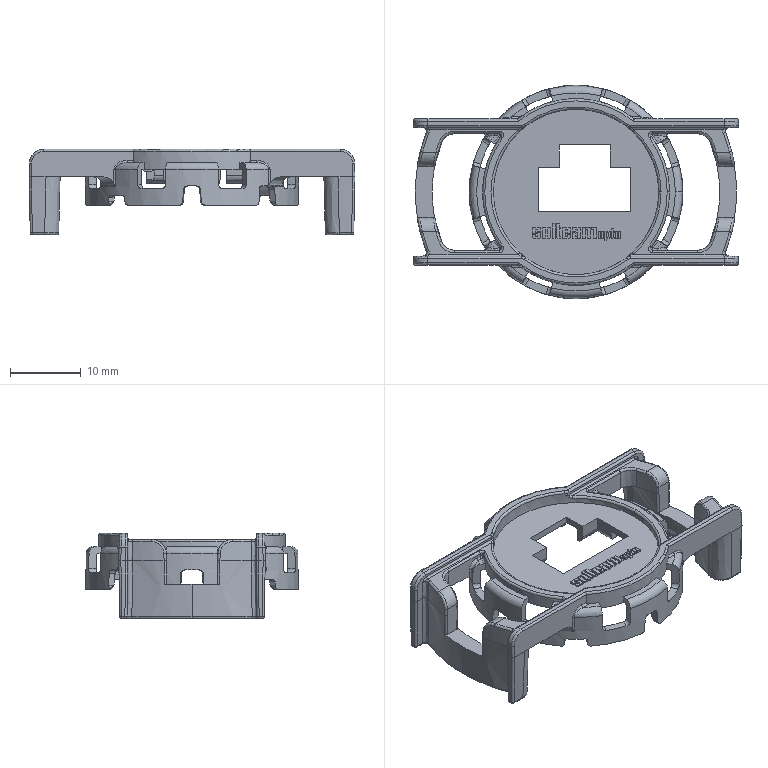Part | STEP file | TBS1006T_P9_W_1 | 1 solid | 774 faces | box 46 x 30.115 x 12.1 mm | volume 2240 mm3 | plane 312 | cylinder 205 | spline 100 | torus 76 | cone 41 | other 22 | sphere 18 | commonest cylinder face diameters 0.6 x88 1 x44 0.403 x23 0.121 x10 0.262 x8 2 x8